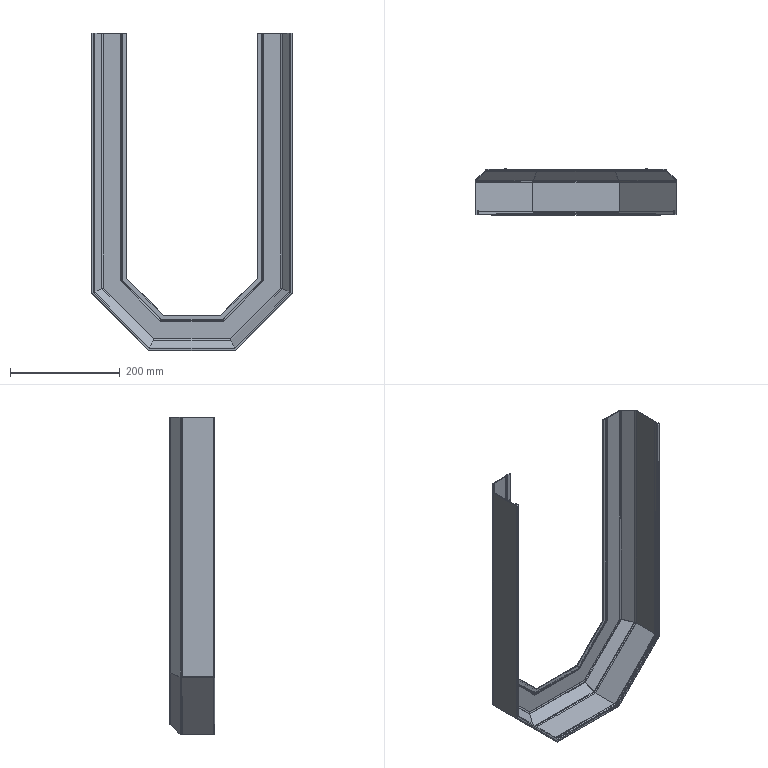Part | STEP file | 51E-01206JG10 | 1 solid | 217 faces | box 367.304 x 82.9 x 577.652 mm | volume 277740 mm3 | cylinder 150 | plane 67 | commonest cylinder face diameters 1 x45 1.8 x30 0.9 x20 0.4 x15 0.6 x10 3 x10